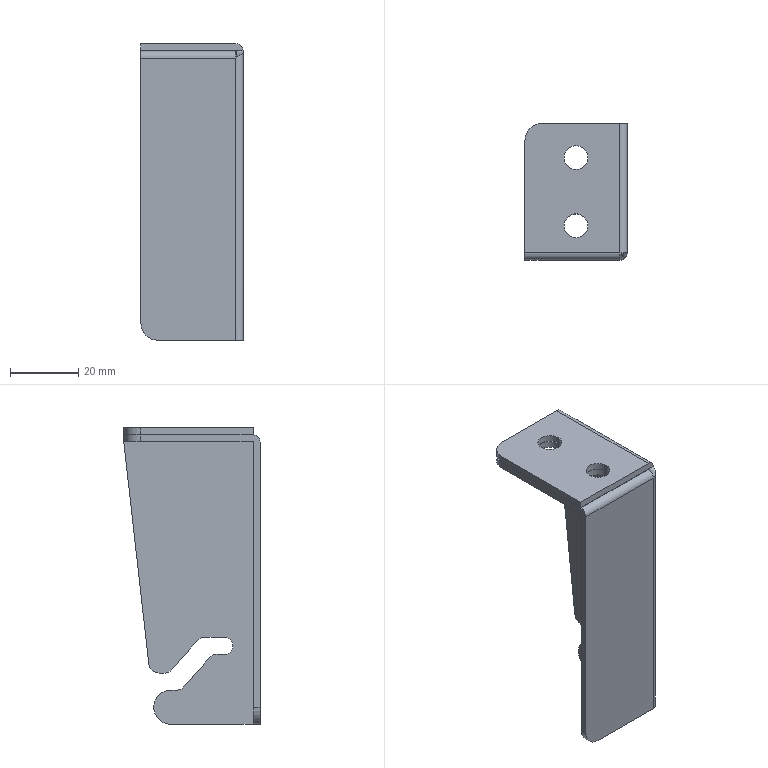Part | STEP file | front lower door bracket-Z (SPCC-3.0) | 1 solid | 47 faces | box 30 x 40 x 87 mm | volume 14354 mm3 | cylinder 24 | plane 22 | spline 1 | commonest cylinder face diameters 7 x8 6 x5 10 x4 0.2 x3 4.2 x3 5 x1